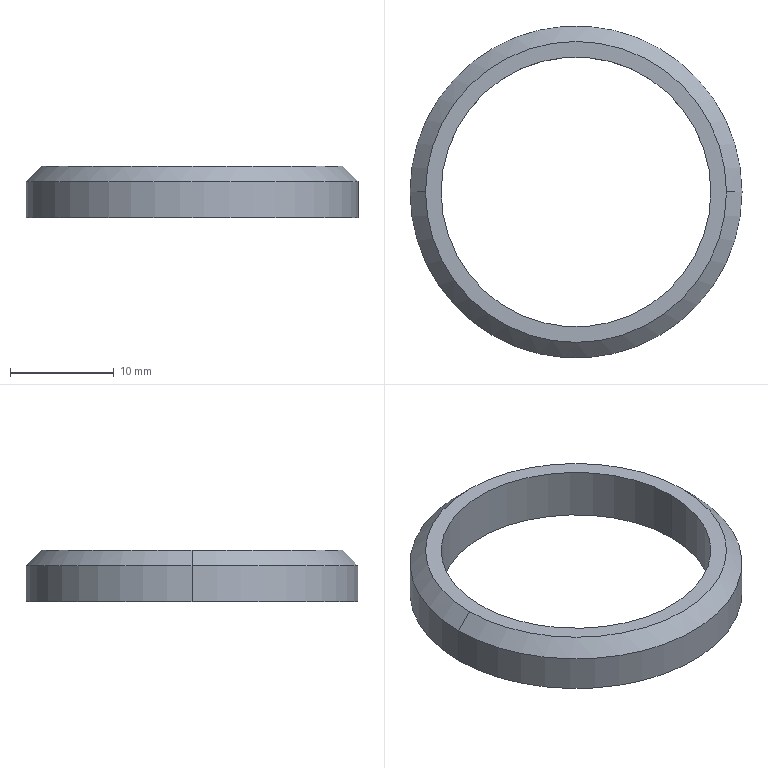Part | SolidWorks | features Chamfer 1, Extrusion 1 | 1 solid | 8 faces | box 32 x 32 x 5 mm | volume 1257 mm3 | cylinder 4 | cone 2 | plane 2 | commonest cylinder face diameters 26 x2 32 x2
STEP:
#1=CARTESIAN_POINT('',(14.5,0.,5.));
#2=VERTEX_POINT('',#1);
#3=CARTESIAN_POINT('',(-14.5,0.,5.));
#4=VERTEX_POINT('',#3);
#5=CARTESIAN_POINT('',(0.,0.,5.));
#6=DIRECTION('',(0.,0.,1.));
#7=DIRECTION('',(1.,0.,0.));
#8=AXIS2_PLACEMENT_3D('',#5,#6,#7);
#9=CIRCLE('',#8,14.5);
#10=EDGE_CURVE('',#2,#4,#9,.T.);
#11=ORIENTED_EDGE('',*,*,#10,.F.);
#12=CARTESIAN_POINT('',(16.,0.,3.5));
#13=VERTEX_POINT('',#12);
#14=CARTESIAN_POINT('',(14.5,0.,5.));
#15=DIRECTION('',(0.7071,0.,-0.7071));
#16=VECTOR('',#15,1000.);
#17=LINE('',#14,#16);
#18=EDGE_CURVE('',#2,#13,#17,.T.);
#19=ORIENTED_EDGE('',*,*,#18,.T.);
#20=CARTESIAN_POINT('',(-16.,0.,3.5));
#21=VERTEX_POINT('',#20);
#22=CARTESIAN_POINT('',(0.,0.,3.5));
#23=DIRECTION('',(0.,0.,-1.));
#24=DIRECTION('',(1.,0.,0.));
#25=AXIS2_PLACEMENT_3D('',#22,#23,#24);
#26=CIRCLE('',#25,16.);
#27=EDGE_CURVE('',#21,#13,#26,.T.);
#28=ORIENTED_EDGE('',*,*,#27,.F.);
#29=CARTESIAN_POINT('',(-14.5,0.,5.));
#30=DIRECTION('',(-0.7071,0.,-0.7071));
#31=VECTOR('',#30,1000.);
#32=LINE('',#29,#31);
#33=EDGE_CURVE('',#4,#21,#32,.T.);
#34=ORIENTED_EDGE('',*,*,#33,.F.);
#35=EDGE_LOOP('',(#11,#19,#28,#34));
#36=FACE_OUTER_BOUND('',#35,.T.);
#37=CARTESIAN_POINT('',(0.,0.,5.));
#38=DIRECTION('',(0.,0.,-1.));
#39=DIRECTION('',(-1.,0.,0.));
#40=AXIS2_PLACEMENT_3D('',#37,#38,#39);
#41=CONICAL_SURFACE('',#40,14.5,0.7854);
#42=ADVANCED_FACE('',(#36),#41,.T.);
#43=CARTESIAN_POINT('',(-13.,0.,5.));
#44=VERTEX_POINT('',#43);
#45=CARTESIAN_POINT('',(13.,0.,5.));
#46=VERTEX_POINT('',#45);
#47=CARTESIAN_POINT('',(0.,0.,5.));
#48=DIRECTION('',(0.,0.,1.));
#49=DIRECTION('',(1.,0.,0.));
#50=AXIS2_PLACEMENT_3D('',#47,#48,#49);
#51=CIRCLE('',#50,13.);
#52=EDGE_CURVE('',#44,#46,#51,.T.);
#53=ORIENTED_EDGE('',*,*,#52,.T.);
#54=CARTESIAN_POINT('',(13.,0.,0.));
#55=VERTEX_POINT('',#54);
#56=CARTESIAN_POINT('',(13.,0.,5.));
#57=DIRECTION('',(0.,0.,-1.));
#58=VECTOR('',#57,1000.);
#59=LINE('',#56,#58);
#60=EDGE_CURVE('',#46,#55,#59,.T.);
#61=ORIENTED_EDGE('',*,*,#60,.T.);
#62=CARTESIAN_POINT('',(-13.,0.,0.));
#63=VERTEX_POINT('',#62);
#64=CARTESIAN_POINT('',(0.,0.,0.));
#65=DIRECTION('',(0.,0.,1.));
#66=DIRECTION('',(1.,0.,0.));
#67=AXIS2_PLACEMENT_3D('',#64,#65,#66);
#68=CIRCLE('',#67,13.);
#69=EDGE_CURVE('',#63,#55,#68,.T.);
#70=ORIENTED_EDGE('',*,*,#69,.F.);
#71=CARTESIAN_POINT('',(-13.,0.,5.));
#72=DIRECTION('',(0.,0.,-1.));
#73=VECTOR('',#72,1000.);
#74=LINE('',#71,#73);
#75=EDGE_CURVE('',#44,#63,#74,.T.);
#76=ORIENTED_EDGE('',*,*,#75,.F.);
#77=EDGE_LOOP('',(#53,#61,#70,#76));
#78=FACE_OUTER_BOUND('',#77,.T.);
#79=CARTESIAN_POINT('',(0.,0.,5.));
#80=DIRECTION('',(0.,0.,-1.));
#81=DIRECTION('',(-1.,0.,0.));
#82=AXIS2_PLACEMENT_3D('',#79,#80,#81);
#83=CYLINDRICAL_SURFACE('',#82,13.);
#84=ADVANCED_FACE('',(#78),#83,.F.);
#85=ORIENTED_EDGE('',*,*,#27,.T.);
#86=CARTESIAN_POINT('',(16.,0.,0.));
#87=VERTEX_POINT('',#86);
#88=CARTESIAN_POINT('',(16.,0.,5.));
#89=DIRECTION('',(0.,0.,-1.));
#90=VECTOR('',#89,1000.);
#91=LINE('',#88,#90);
#92=EDGE_CURVE('',#13,#87,#91,.T.);
#93=ORIENTED_EDGE('',*,*,#92,.T.);
#94=CARTESIAN_POINT('',(-16.,0.,0.));
#95=VERTEX_POINT('',#94);
#96=CARTESIAN_POINT('',(0.,0.,0.));
#97=DIRECTION('',(0.,0.,1.));
#98=DIRECTION('',(1.,0.,0.));
#99=AXIS2_PLACEMENT_3D('',#96,#97,#98);
#100=CIRCLE('',#99,16.);
#101=EDGE_CURVE('',#87,#95,#100,.T.);
#102=ORIENTED_EDGE('',*,*,#101,.T.);
#103=CARTESIAN_POINT('',(-16.,0.,5.));
#104=DIRECTION('',(0.,0.,-1.));
#105=VECTOR('',#104,1000.);
#106=LINE('',#103,#105);
#107=EDGE_CURVE('',#21,#95,#106,.T.);
#108=ORIENTED_EDGE('',*,*,#107,.F.);
#109=EDGE_LOOP('',(#85,#93,#102,#108));
#110=FACE_OUTER_BOUND('',#109,.T.);
#111=CARTESIAN_POINT('',(0.,0.,5.));
#112=DIRECTION('',(0.,0.,-1.));
#113=DIRECTION('',(-1.,0.,0.));
#114=AXIS2_PLACEMENT_3D('',#111,#112,#113);
#115=CYLINDRICAL_SURFACE('',#114,16.);
#116=ADVANCED_FACE('',(#110),#115,.T.);
#117=CARTESIAN_POINT('',(0.,0.,5.));
#118=DIRECTION('',(0.,0.,1.));
#119=DIRECTION('',(1.,0.,0.));
#120=AXIS2_PLACEMENT_3D('',#117,#118,#119);
#121=CIRCLE('',#120,14.5);
#122=EDGE_CURVE('',#4,#2,#121,.T.);
#123=ORIENTED_EDGE('',*,*,#122,.T.);
#124=ORIENTED_EDGE('',*,*,#10,.T.);
#125=EDGE_LOOP('',(#123,#124));
#126=FACE_OUTER_BOUND('',#125,.T.);
#127=ORIENTED_EDGE('',*,*,#52,.F.);
#128=CARTESIAN_POINT('',(0.,0.,5.));
#129=DIRECTION('',(0.,0.,1.));
#130=DIRECTION('',(1.,0.,0.));
#131=AXIS2_PLACEMENT_3D('',#128,#129,#130);
#132=CIRCLE('',#131,13.);
#133=EDGE_CURVE('',#46,#44,#132,.T.);
#134=ORIENTED_EDGE('',*,*,#133,.F.);
#135=EDGE_LOOP('',(#127,#134));
#136=FACE_BOUND('',#135,.T.);
#137=CARTESIAN_POINT('',(0.,0.,5.));
#138=DIRECTION('',(0.,0.,1.));
#139=DIRECTION('',(1.,0.,0.));
#140=AXIS2_PLACEMENT_3D('',#137,#138,#139);
#141=PLANE('',#140);
#142=ADVANCED_FACE('',(#126,#136),#141,.T.);
#143=CARTESIAN_POINT('',(0.,0.,0.));
#144=DIRECTION('',(0.,0.,1.));
#145=DIRECTION('',(1.,0.,0.));
#146=AXIS2_PLACEMENT_3D('',#143,#144,#145);
#147=CIRCLE('',#146,16.);
#148=EDGE_CURVE('',#95,#87,#147,.T.);
#149=ORIENTED_EDGE('',*,*,#148,.F.);
#150=ORIENTED_EDGE('',*,*,#101,.F.);
#151=EDGE_LOOP('',(#149,#150));
#152=FACE_OUTER_BOUND('',#151,.T.);
#153=ORIENTED_EDGE('',*,*,#69,.T.);
#154=CARTESIAN_POINT('',(0.,0.,0.));
#155=DIRECTION('',(0.,0.,1.));
#156=DIRECTION('',(1.,0.,0.));
#157=AXIS2_PLACEMENT_3D('',#154,#155,#156);
#158=CIRCLE('',#157,13.);
#159=EDGE_CURVE('',#55,#63,#158,.T.);
#160=ORIENTED_EDGE('',*,*,#159,.T.);
#161=EDGE_LOOP('',(#153,#160));
#162=FACE_BOUND('',#161,.T.);
#163=CARTESIAN_POINT('',(0.,0.,0.));
#164=DIRECTION('',(0.,0.,1.));
#165=DIRECTION('',(1.,0.,0.));
#166=AXIS2_PLACEMENT_3D('',#163,#164,#165);
#167=PLANE('',#166);
#168=ADVANCED_FACE('',(#152,#162),#167,.F.);
#169=ORIENTED_EDGE('',*,*,#92,.F.);
#170=CARTESIAN_POINT('',(0.,0.,3.5));
#171=DIRECTION('',(0.,0.,-1.));
#172=DIRECTION('',(1.,0.,0.));
#173=AXIS2_PLACEMENT_3D('',#170,#171,#172);
#174=CIRCLE('',#173,16.);
#175=EDGE_CURVE('',#13,#21,#174,.T.);
#176=ORIENTED_EDGE('',*,*,#175,.T.);
#177=ORIENTED_EDGE('',*,*,#107,.T.);
#178=ORIENTED_EDGE('',*,*,#148,.T.);
#179=EDGE_LOOP('',(#169,#176,#177,#178));
#180=FACE_OUTER_BOUND('',#179,.T.);
#181=CARTESIAN_POINT('',(0.,0.,5.));
#182=DIRECTION('',(0.,0.,-1.));
#183=DIRECTION('',(-1.,0.,0.));
#184=AXIS2_PLACEMENT_3D('',#181,#182,#183);
#185=CYLINDRICAL_SURFACE('',#184,16.);
#186=ADVANCED_FACE('',(#180),#185,.T.);
#187=ORIENTED_EDGE('',*,*,#60,.F.);
#188=ORIENTED_EDGE('',*,*,#133,.T.);
#189=ORIENTED_EDGE('',*,*,#75,.T.);
#190=ORIENTED_EDGE('',*,*,#159,.F.);
#191=EDGE_LOOP('',(#187,#188,#189,#190));
#192=FACE_OUTER_BOUND('',#191,.T.);
#193=CARTESIAN_POINT('',(0.,0.,5.));
#194=DIRECTION('',(0.,0.,-1.));
#195=DIRECTION('',(-1.,0.,0.));
#196=AXIS2_PLACEMENT_3D('',#193,#194,#195);
#197=CYLINDRICAL_SURFACE('',#196,13.);
#198=ADVANCED_FACE('',(#192),#197,.F.);
#199=ORIENTED_EDGE('',*,*,#18,.F.);
#200=ORIENTED_EDGE('',*,*,#122,.F.);
#201=ORIENTED_EDGE('',*,*,#33,.T.);
#202=ORIENTED_EDGE('',*,*,#175,.F.);
#203=EDGE_LOOP('',(#199,#200,#201,#202));
#204=FACE_OUTER_BOUND('',#203,.T.);
#205=CARTESIAN_POINT('',(0.,0.,5.));
#206=DIRECTION('',(0.,0.,-1.));
#207=DIRECTION('',(-1.,0.,0.));
#208=AXIS2_PLACEMENT_3D('',#205,#206,#207);
#209=CONICAL_SURFACE('',#208,14.5,0.7854);
#210=ADVANCED_FACE('',(#204),#209,.T.);
#211=CLOSED_SHELL('',(#42,#84,#116,#142,#168,#186,#198,#210));
#212=MANIFOLD_SOLID_BREP('',#211);
#213=CARTESIAN_POINT('',(0.,0.,0.));
#214=DIRECTION('',(0.,0.,1.));
#215=DIRECTION('',(1.,0.,0.));
#216=AXIS2_PLACEMENT_3D('',#213,#214,#215);
#217=(LENGTH_UNIT()NAMED_UNIT(*)SI_UNIT(.MILLI.,.METRE.));
#218=UNCERTAINTY_MEASURE_WITH_UNIT(LENGTH_MEASURE(0.00001),#217,'','');
#219=(NAMED_UNIT(*)PLANE_ANGLE_UNIT()SI_UNIT($,.RADIAN.));
#220=(NAMED_UNIT(*)SI_UNIT($,.STERADIAN.)SOLID_ANGLE_UNIT());
#221=(GEOMETRIC_REPRESENTATION_CONTEXT(3)GLOBAL_UNCERTAINTY_ASSIGNED_CONTEXT((#218))GLOBAL_UNIT_ASSIGNED_CONTEXT((#217,#219,#220))REPRESENTATION_CONTEXT('',''));
#222=ADVANCED_BREP_SHAPE_REPRESENTATION('',(#212,#216),#221);